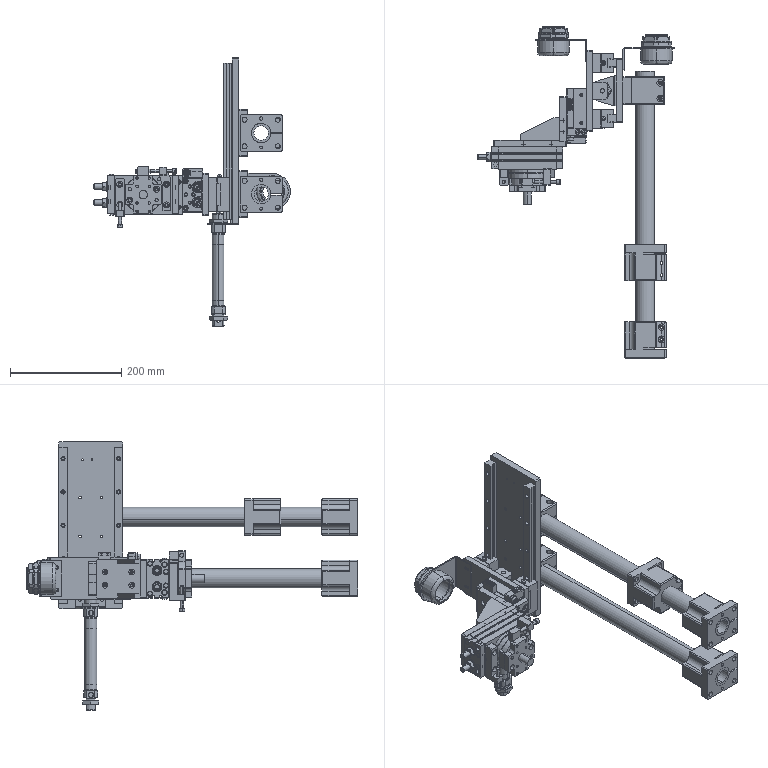Part | SolidWorks | 46 solids | 2645 faces | box 353.5 x 596.5 x 482 mm | volume 3186701 mm3 | cylinder 1102 | plane 1085 | cone 398 | spline 38 | torus 22 | commonest cylinder face diameters 4 x108 9 x65 5 x57 4.5 x56 4.917 x54 8 x44